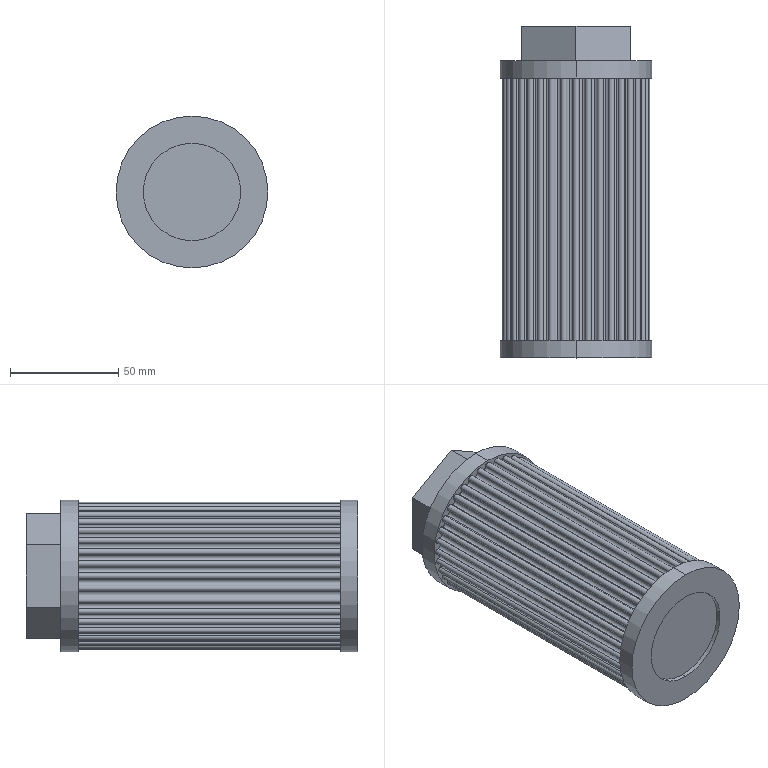Part | SolidWorks | features ICE 2, Revolution 1, SweepThread 1 | 1 solid | 147 faces | box 70 x 153 x 70 mm | volume 294269 mm3 | cylinder 129 | plane 15 | spline 3 | commonest cylinder face diameters 2.835 x111 42 x12 70 x4 45 x2